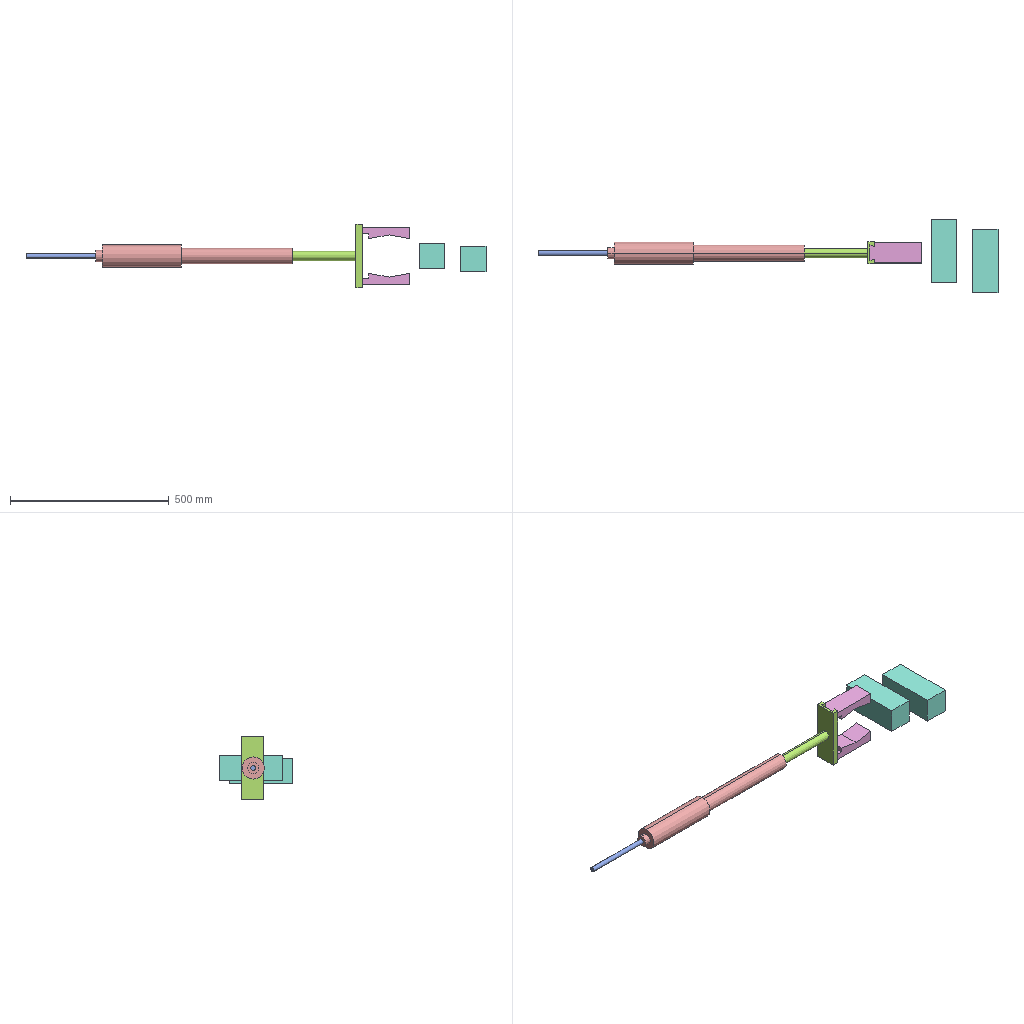Assembly | SolidWorks | 7 different items | 9 placed | box 1450 x 230 x 200 mm
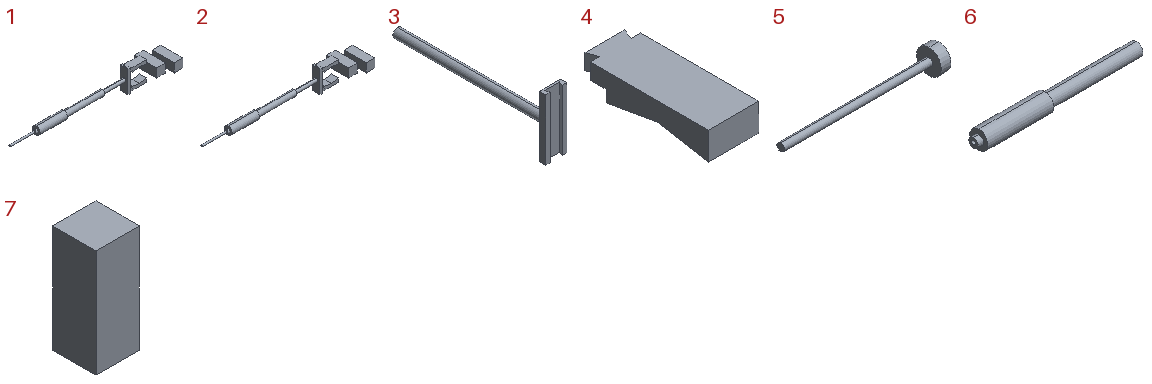Parts list (item | name | quantity | size | volume | features):
1 | (subassembly) | x1 | 1450 x 230 x 200 mm | 4682251 mm3 | features AEMSimFeature 1
2 | (subassembly) | x1 | 1450 x 230 x 200 mm | 4682251 mm3 | features AEMSimFeature 1
3 | - | x1 | 70 x 520 x 200 mm | 509793 mm3 | features Extrusion 1, ICE 1
4 | - | x2 | 64 x 163.737 x 35 mm | 281485 mm3 | features Extrusion 1, ICE 1
5 | - | x1 | 320 x 50 x 50 mm | 92284 mm3 | features Revolution 1
6 | - | x1 | 620 x 70 x 70 mm | 957204 mm3 | features Revolution 1
7 | - | x2 | 80 x 80 x 200 mm | 1280000 mm3 | features Extrusion 1
Mates (type | each side: item.copy, entity, surface, feature):
Concentric | 6.1 face cylinder Revolve1 | 5.1 face cylinder Revolve1
Concentric | 6.1 face cylinder Revolve1 | 3.1 face cylinder Boss-Extrude2
Parallel | 3.1 face plane Boss-Extrude1 | assembly plane
Coincident | 3.1 face plane Boss-Extrude1 | 4.1 face plane Boss-Extrude1 | 2 times
Coincident | 3.1 face plane Boss-Extrude1 | 4.2 face plane Boss-Extrude1 | 2 times